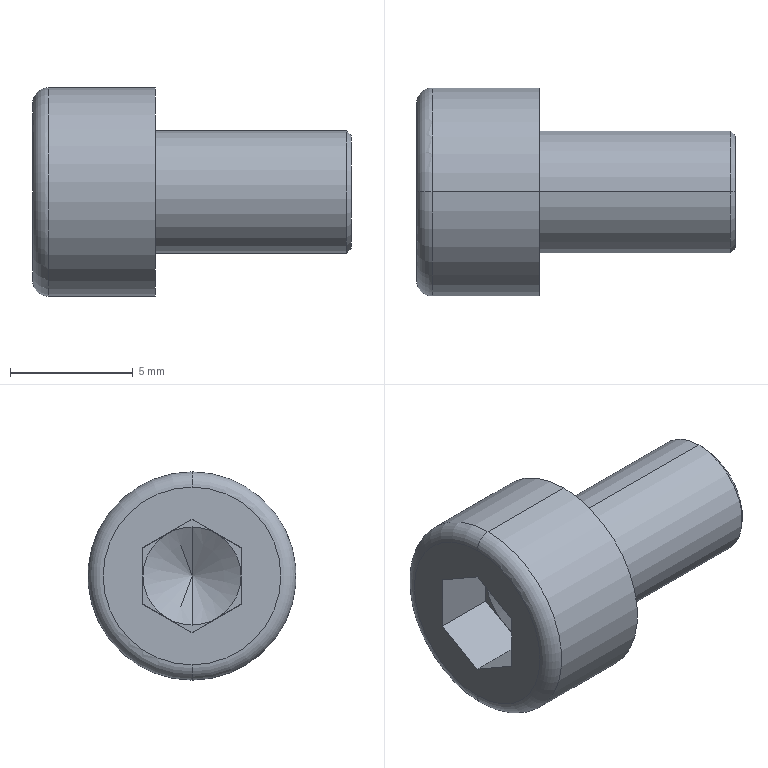Part | STEP file | hexagon socket head cap screws gb_GB_FASTENER_SCREWS_HSHCS M5X8-C | 1 solid | 25 faces | box 13 x 8.5 x 8.5 mm | volume 398.856 mm3 | plane 15 | cone 4 | cylinder 4 | torus 2 | commonest cylinder face diameters 5 x2 8.5 x2
STEP:
#1=CARTESIAN_POINT('',(13.,0.,-2.3));
#2=VERTEX_POINT('',#1);
#3=CARTESIAN_POINT('',(13.,0.,2.3));
#4=VERTEX_POINT('',#3);
#5=CARTESIAN_POINT('',(13.,0.,0.));
#6=DIRECTION('',(1.,0.,0.));
#7=DIRECTION('',(0.,0.,-1.));
#8=AXIS2_PLACEMENT_3D('',#5,#6,#7);
#9=CIRCLE('',#8,2.3);
#10=EDGE_CURVE('',#2,#4,#9,.T.);
#11=ORIENTED_EDGE('',*,*,#10,.F.);
#12=CARTESIAN_POINT('',(12.8,0.,-2.5));
#13=VERTEX_POINT('',#12);
#14=CARTESIAN_POINT('',(13.,0.,-2.3));
#15=DIRECTION('',(-0.7071,0.,-0.7071));
#16=VECTOR('',#15,1000.);
#17=LINE('',#14,#16);
#18=EDGE_CURVE('',#2,#13,#17,.T.);
#19=ORIENTED_EDGE('',*,*,#18,.T.);
#20=CARTESIAN_POINT('',(12.8,0.,2.5));
#21=VERTEX_POINT('',#20);
#22=CARTESIAN_POINT('',(12.8,0.,0.));
#23=DIRECTION('',(-1.,0.,0.));
#24=DIRECTION('',(0.,0.,-1.));
#25=AXIS2_PLACEMENT_3D('',#22,#23,#24);
#26=CIRCLE('',#25,2.5);
#27=EDGE_CURVE('',#21,#13,#26,.T.);
#28=ORIENTED_EDGE('',*,*,#27,.F.);
#29=CARTESIAN_POINT('',(13.,0.,2.3));
#30=DIRECTION('',(-0.7071,0.,0.7071));
#31=VECTOR('',#30,1000.);
#32=LINE('',#29,#31);
#33=EDGE_CURVE('',#4,#21,#32,.T.);
#34=ORIENTED_EDGE('',*,*,#33,.F.);
#35=EDGE_LOOP('',(#11,#19,#28,#34));
#36=FACE_OUTER_BOUND('',#35,.T.);
#37=CARTESIAN_POINT('',(13.,0.,0.));
#38=DIRECTION('',(-1.,0.,0.));
#39=DIRECTION('',(0.,0.,1.));
#40=AXIS2_PLACEMENT_3D('',#37,#38,#39);
#41=CONICAL_SURFACE('',#40,2.3,0.7854);
#42=ADVANCED_FACE('',(#36),#41,.T.);
#43=CARTESIAN_POINT('',(0.,0.,3.625));
#44=VERTEX_POINT('',#43);
#45=CARTESIAN_POINT('',(0.,0.,-3.625));
#46=VERTEX_POINT('',#45);
#47=CARTESIAN_POINT('',(0.,0.,0.));
#48=DIRECTION('',(-1.,0.,0.));
#49=DIRECTION('',(0.,0.,-1.));
#50=AXIS2_PLACEMENT_3D('',#47,#48,#49);
#51=CIRCLE('',#50,3.625);
#52=EDGE_CURVE('',#44,#46,#51,.T.);
#53=ORIENTED_EDGE('',*,*,#52,.F.);
#54=CARTESIAN_POINT('',(0.625,0.,4.25));
#55=VERTEX_POINT('',#54);
#56=CARTESIAN_POINT('',(0.625,0.,3.625));
#57=DIRECTION('',(0.,1.,0.));
#58=DIRECTION('',(0.,0.,1.));
#59=AXIS2_PLACEMENT_3D('',#56,#57,#58);
#60=CIRCLE('',#59,0.625);
#61=EDGE_CURVE('',#44,#55,#60,.T.);
#62=ORIENTED_EDGE('',*,*,#61,.T.);
#63=CARTESIAN_POINT('',(0.625,0.,-4.25));
#64=VERTEX_POINT('',#63);
#65=CARTESIAN_POINT('',(0.625,0.,0.));
#66=DIRECTION('',(1.,0.,0.));
#67=DIRECTION('',(0.,0.,-1.));
#68=AXIS2_PLACEMENT_3D('',#65,#66,#67);
#69=CIRCLE('',#68,4.25);
#70=EDGE_CURVE('',#64,#55,#69,.T.);
#71=ORIENTED_EDGE('',*,*,#70,.F.);
#72=CARTESIAN_POINT('',(0.625,0.,-3.625));
#73=DIRECTION('',(0.,-1.,0.));
#74=DIRECTION('',(0.,0.,-1.));
#75=AXIS2_PLACEMENT_3D('',#72,#73,#74);
#76=CIRCLE('',#75,0.625);
#77=EDGE_CURVE('',#46,#64,#76,.T.);
#78=ORIENTED_EDGE('',*,*,#77,.F.);
#79=EDGE_LOOP('',(#53,#62,#71,#78));
#80=FACE_OUTER_BOUND('',#79,.T.);
#81=CARTESIAN_POINT('',(0.625,0.,0.));
#82=DIRECTION('',(1.,0.,0.));
#83=DIRECTION('',(0.,0.,-1.));
#84=AXIS2_PLACEMENT_3D('',#81,#82,#83);
#85=TOROIDAL_SURFACE('',#84,3.625,0.625);
#86=ADVANCED_FACE('',(#80),#85,.T.);
#87=CARTESIAN_POINT('',(3.655,0.,0.));
#88=VERTEX_POINT('',#87);
#89=CARTESIAN_POINT('',(2.5,0.,2.));
#90=VERTEX_POINT('',#89);
#91=CARTESIAN_POINT('',(2.5,0.,2.));
#92=DIRECTION('',(-0.5,0.,0.866));
#93=VECTOR('',#92,1000.);
#94=LINE('',#91,#93);
#95=EDGE_CURVE('',#88,#90,#94,.T.);
#96=ORIENTED_EDGE('',*,*,#95,.F.);
#97=CARTESIAN_POINT('',(2.5,0.,-2.));
#98=VERTEX_POINT('',#97);
#99=CARTESIAN_POINT('',(2.5,0.,-2.));
#100=DIRECTION('',(-0.5,0.,-0.866));
#101=VECTOR('',#100,1000.);
#102=LINE('',#99,#101);
#103=EDGE_CURVE('',#88,#98,#102,.T.);
#104=ORIENTED_EDGE('',*,*,#103,.T.);
#105=CARTESIAN_POINT('',(2.5,-1.,-1.732));
#106=VERTEX_POINT('',#105);
#107=CARTESIAN_POINT('',(2.5,0.,0.));
#108=DIRECTION('',(-1.,0.,0.));
#109=DIRECTION('',(0.,0.,-1.));
#110=AXIS2_PLACEMENT_3D('',#107,#108,#109);
#111=CIRCLE('',#110,2.);
#112=EDGE_CURVE('',#98,#106,#111,.T.);
#113=ORIENTED_EDGE('',*,*,#112,.T.);
#114=CARTESIAN_POINT('',(2.5,-2.,0.));
#115=VERTEX_POINT('',#114);
#116=CARTESIAN_POINT('',(2.5,0.,0.));
#117=DIRECTION('',(-1.,0.,0.));
#118=DIRECTION('',(0.,0.,-1.));
#119=AXIS2_PLACEMENT_3D('',#116,#117,#118);
#120=CIRCLE('',#119,2.);
#121=EDGE_CURVE('',#106,#115,#120,.T.);
#122=ORIENTED_EDGE('',*,*,#121,.T.);
#123=CARTESIAN_POINT('',(2.5,-1.,1.732));
#124=VERTEX_POINT('',#123);
#125=CARTESIAN_POINT('',(2.5,0.,0.));
#126=DIRECTION('',(-1.,0.,0.));
#127=DIRECTION('',(0.,0.,-1.));
#128=AXIS2_PLACEMENT_3D('',#125,#126,#127);
#129=CIRCLE('',#128,2.);
#130=EDGE_CURVE('',#115,#124,#129,.T.);
#131=ORIENTED_EDGE('',*,*,#130,.T.);
#132=CARTESIAN_POINT('',(2.5,0.,0.));
#133=DIRECTION('',(-1.,0.,0.));
#134=DIRECTION('',(0.,0.,-1.));
#135=AXIS2_PLACEMENT_3D('',#132,#133,#134);
#136=CIRCLE('',#135,2.);
#137=EDGE_CURVE('',#124,#90,#136,.T.);
#138=ORIENTED_EDGE('',*,*,#137,.T.);
#139=EDGE_LOOP('',(#96,#104,#113,#122,#131,#138));
#140=FACE_OUTER_BOUND('',#139,.T.);
#141=CARTESIAN_POINT('',(2.5,0.,0.));
#142=DIRECTION('',(-1.,0.,0.));
#143=DIRECTION('',(0.,0.,1.));
#144=AXIS2_PLACEMENT_3D('',#141,#142,#143);
#145=CONICAL_SURFACE('',#144,2.,1.047);
#146=ADVANCED_FACE('',(#140),#145,.F.);
#147=ORIENTED_EDGE('',*,*,#27,.T.);
#148=CARTESIAN_POINT('',(5.,0.,-2.5));
#149=VERTEX_POINT('',#148);
#150=CARTESIAN_POINT('',(13.,0.,-2.5));
#151=DIRECTION('',(-1.,0.,0.));
#152=VECTOR('',#151,1000.);
#153=LINE('',#150,#152);
#154=EDGE_CURVE('',#13,#149,#153,.T.);
#155=ORIENTED_EDGE('',*,*,#154,.T.);
#156=CARTESIAN_POINT('',(5.,0.,2.5));
#157=VERTEX_POINT('',#156);
#158=CARTESIAN_POINT('',(5.,0.,0.));
#159=DIRECTION('',(1.,0.,0.));
#160=DIRECTION('',(0.,0.,-1.));
#161=AXIS2_PLACEMENT_3D('',#158,#159,#160);
#162=CIRCLE('',#161,2.5);
#163=EDGE_CURVE('',#149,#157,#162,.T.);
#164=ORIENTED_EDGE('',*,*,#163,.T.);
#165=CARTESIAN_POINT('',(13.,0.,2.5));
#166=DIRECTION('',(-1.,0.,0.));
#167=VECTOR('',#166,1000.);
#168=LINE('',#165,#167);
#169=EDGE_CURVE('',#21,#157,#168,.T.);
#170=ORIENTED_EDGE('',*,*,#169,.F.);
#171=EDGE_LOOP('',(#147,#155,#164,#170));
#172=FACE_OUTER_BOUND('',#171,.T.);
#173=CARTESIAN_POINT('',(13.,0.,0.));
#174=DIRECTION('',(-1.,0.,0.));
#175=DIRECTION('',(0.,0.,1.));
#176=AXIS2_PLACEMENT_3D('',#173,#174,#175);
#177=CYLINDRICAL_SURFACE('',#176,2.5);
#178=ADVANCED_FACE('',(#172),#177,.T.);
#179=CARTESIAN_POINT('',(5.,0.,-4.25));
#180=VERTEX_POINT('',#179);
#181=CARTESIAN_POINT('',(5.,0.,4.25));
#182=VERTEX_POINT('',#181);
#183=CARTESIAN_POINT('',(5.,0.,0.));
#184=DIRECTION('',(1.,0.,0.));
#185=DIRECTION('',(0.,0.,-1.));
#186=AXIS2_PLACEMENT_3D('',#183,#184,#185);
#187=CIRCLE('',#186,4.25);
#188=EDGE_CURVE('',#180,#182,#187,.T.);
#189=ORIENTED_EDGE('',*,*,#188,.F.);
#190=CARTESIAN_POINT('',(5.,0.,-4.25));
#191=DIRECTION('',(-1.,0.,0.));
#192=VECTOR('',#191,1000.);
#193=LINE('',#190,#192);
#194=EDGE_CURVE('',#180,#64,#193,.T.);
#195=ORIENTED_EDGE('',*,*,#194,.T.);
#196=ORIENTED_EDGE('',*,*,#70,.T.);
#197=CARTESIAN_POINT('',(5.,0.,4.25));
#198=DIRECTION('',(-1.,0.,0.));
#199=VECTOR('',#198,1000.);
#200=LINE('',#197,#199);
#201=EDGE_CURVE('',#182,#55,#200,.T.);
#202=ORIENTED_EDGE('',*,*,#201,.F.);
#203=EDGE_LOOP('',(#189,#195,#196,#202));
#204=FACE_OUTER_BOUND('',#203,.T.);
#205=CARTESIAN_POINT('',(5.,0.,0.));
#206=DIRECTION('',(-1.,0.,0.));
#207=DIRECTION('',(0.,0.,1.));
#208=AXIS2_PLACEMENT_3D('',#205,#206,#207);
#209=CYLINDRICAL_SURFACE('',#208,4.25);
#210=ADVANCED_FACE('',(#204),#209,.T.);
#211=ORIENTED_EDGE('',*,*,#121,.F.);
#212=CARTESIAN_POINT('',(2.5,-2.,-1.155));
#213=VERTEX_POINT('',#212);
#214=CARTESIAN_POINT('',(2.5,-2.,-1.155));
#215=DIRECTION('',(0.,0.866,-0.5));
#216=VECTOR('',#215,1000.);
#217=LINE('',#214,#216);
#218=EDGE_CURVE('',#213,#106,#217,.T.);
#219=ORIENTED_EDGE('',*,*,#218,.F.);
#220=CARTESIAN_POINT('',(2.5,-2.,1.155));
#221=DIRECTION('',(0.,0.,-1.));
#222=VECTOR('',#221,1000.);
#223=LINE('',#220,#222);
#224=EDGE_CURVE('',#115,#213,#223,.T.);
#225=ORIENTED_EDGE('',*,*,#224,.F.);
#226=EDGE_LOOP('',(#211,#219,#225));
#227=FACE_OUTER_BOUND('',#226,.T.);
#228=CARTESIAN_POINT('',(2.5,0.,-2.309));
#229=DIRECTION('',(1.,0.,0.));
#230=DIRECTION('',(0.,0.,-1.));
#231=AXIS2_PLACEMENT_3D('',#228,#229,#230);
#232=PLANE('',#231);
#233=ADVANCED_FACE('',(#227),#232,.F.);
#234=ORIENTED_EDGE('',*,*,#130,.F.);
#235=CARTESIAN_POINT('',(2.5,-2.,1.155));
#236=VERTEX_POINT('',#235);
#237=CARTESIAN_POINT('',(2.5,-2.,1.155));
#238=DIRECTION('',(0.,0.,-1.));
#239=VECTOR('',#238,1000.);
#240=LINE('',#237,#239);
#241=EDGE_CURVE('',#236,#115,#240,.T.);
#242=ORIENTED_EDGE('',*,*,#241,.F.);
#243=CARTESIAN_POINT('',(2.5,0.,2.309));
#244=DIRECTION('',(0.,-0.866,-0.5));
#245=VECTOR('',#244,1000.);
#246=LINE('',#243,#245);
#247=EDGE_CURVE('',#124,#236,#246,.T.);
#248=ORIENTED_EDGE('',*,*,#247,.F.);
#249=EDGE_LOOP('',(#234,#242,#248));
#250=FACE_OUTER_BOUND('',#249,.T.);
#251=CARTESIAN_POINT('',(2.5,0.,-2.309));
#252=DIRECTION('',(1.,0.,0.));
#253=DIRECTION('',(0.,0.,-1.));
#254=AXIS2_PLACEMENT_3D('',#251,#252,#253);
#255=PLANE('',#254);
#256=ADVANCED_FACE('',(#250),#255,.F.);
#257=ORIENTED_EDGE('',*,*,#137,.F.);
#258=CARTESIAN_POINT('',(2.5,0.,2.309));
#259=VERTEX_POINT('',#258);
#260=CARTESIAN_POINT('',(2.5,0.,2.309));
#261=DIRECTION('',(0.,-0.866,-0.5));
#262=VECTOR('',#261,1000.);
#263=LINE('',#260,#262);
#264=EDGE_CURVE('',#259,#124,#263,.T.);
#265=ORIENTED_EDGE('',*,*,#264,.F.);
#266=CARTESIAN_POINT('',(2.5,1.,1.732));
#267=VERTEX_POINT('',#266);
#268=CARTESIAN_POINT('',(2.5,2.,1.155));
#269=DIRECTION('',(0.,-0.866,0.5));
#270=VECTOR('',#269,1000.);
#271=LINE('',#268,#270);
#272=EDGE_CURVE('',#267,#259,#271,.T.);
#273=ORIENTED_EDGE('',*,*,#272,.F.);
#274=CARTESIAN_POINT('',(2.5,0.,0.));
#275=DIRECTION('',(-1.,0.,0.));
#276=DIRECTION('',(0.,0.,-1.));
#277=AXIS2_PLACEMENT_3D('',#274,#275,#276);
#278=CIRCLE('',#277,2.);
#279=EDGE_CURVE('',#90,#267,#278,.T.);
#280=ORIENTED_EDGE('',*,*,#279,.F.);
#281=EDGE_LOOP('',(#257,#265,#273,#280));
#282=FACE_OUTER_BOUND('',#281,.T.);
#283=CARTESIAN_POINT('',(2.5,0.,-2.309));
#284=DIRECTION('',(1.,0.,0.));
#285=DIRECTION('',(0.,0.,-1.));
#286=AXIS2_PLACEMENT_3D('',#283,#284,#285);
#287=PLANE('',#286);
#288=ADVANCED_FACE('',(#282),#287,.F.);
#289=CARTESIAN_POINT('',(2.5,2.,0.));
#290=VERTEX_POINT('',#289);
#291=CARTESIAN_POINT('',(2.5,0.,0.));
#292=DIRECTION('',(-1.,0.,0.));
#293=DIRECTION('',(0.,0.,-1.));
#294=AXIS2_PLACEMENT_3D('',#291,#292,#293);
#295=CIRCLE('',#294,2.);
#296=EDGE_CURVE('',#267,#290,#295,.T.);
#297=ORIENTED_EDGE('',*,*,#296,.F.);
#298=CARTESIAN_POINT('',(2.5,2.,1.155));
#299=VERTEX_POINT('',#298);
#300=CARTESIAN_POINT('',(2.5,2.,1.155));
#301=DIRECTION('',(0.,-0.866,0.5));
#302=VECTOR('',#301,1000.);
#303=LINE('',#300,#302);
#304=EDGE_CURVE('',#299,#267,#303,.T.);
#305=ORIENTED_EDGE('',*,*,#304,.F.);
#306=CARTESIAN_POINT('',(2.5,2.,-1.155));
#307=DIRECTION('',(0.,0.,1.));
#308=VECTOR('',#307,1000.);
#309=LINE('',#306,#308);
#310=EDGE_CURVE('',#290,#299,#309,.T.);
#311=ORIENTED_EDGE('',*,*,#310,.F.);
#312=EDGE_LOOP('',(#297,#305,#311));
#313=FACE_OUTER_BOUND('',#312,.T.);
#314=CARTESIAN_POINT('',(2.5,0.,-2.309));
#315=DIRECTION('',(1.,0.,0.));
#316=DIRECTION('',(0.,0.,-1.));
#317=AXIS2_PLACEMENT_3D('',#314,#315,#316);
#318=PLANE('',#317);
#319=ADVANCED_FACE('',(#313),#318,.F.);
#320=CARTESIAN_POINT('',(2.5,1.,-1.732));
#321=VERTEX_POINT('',#320);
#322=CARTESIAN_POINT('',(2.5,0.,0.));
#323=DIRECTION('',(1.,0.,0.));
#324=DIRECTION('',(0.,0.,-1.));
#325=AXIS2_PLACEMENT_3D('',#322,#323,#324);
#326=CIRCLE('',#325,2.);
#327=EDGE_CURVE('',#321,#290,#326,.T.);
#328=ORIENTED_EDGE('',*,*,#327,.T.);
#329=CARTESIAN_POINT('',(2.5,2.,-1.155));
#330=VERTEX_POINT('',#329);
#331=CARTESIAN_POINT('',(2.5,2.,-1.155));
#332=DIRECTION('',(0.,0.,1.));
#333=VECTOR('',#332,1000.);
#334=LINE('',#331,#333);
#335=EDGE_CURVE('',#330,#290,#334,.T.);
#336=ORIENTED_EDGE('',*,*,#335,.F.);
#337=CARTESIAN_POINT('',(2.5,0.,-2.309));
#338=DIRECTION('',(0.,0.866,0.5));
#339=VECTOR('',#338,1000.);
#340=LINE('',#337,#339);
#341=EDGE_CURVE('',#321,#330,#340,.T.);
#342=ORIENTED_EDGE('',*,*,#341,.F.);
#343=EDGE_LOOP('',(#328,#336,#342));
#344=FACE_OUTER_BOUND('',#343,.T.);
#345=CARTESIAN_POINT('',(2.5,0.,-2.309));
#346=DIRECTION('',(1.,0.,0.));
#347=DIRECTION('',(0.,0.,-1.));
#348=AXIS2_PLACEMENT_3D('',#345,#346,#347);
#349=PLANE('',#348);
#350=ADVANCED_FACE('',(#344),#349,.F.);
#351=CARTESIAN_POINT('',(2.5,0.,0.));
#352=DIRECTION('',(-1.,0.,0.));
#353=DIRECTION('',(0.,0.,-1.));
#354=AXIS2_PLACEMENT_3D('',#351,#352,#353);
#355=CIRCLE('',#354,2.);
#356=EDGE_CURVE('',#321,#98,#355,.T.);
#357=ORIENTED_EDGE('',*,*,#356,.F.);
#358=CARTESIAN_POINT('',(2.5,0.,-2.309));
#359=VERTEX_POINT('',#358);
#360=CARTESIAN_POINT('',(2.5,0.,-2.309));
#361=DIRECTION('',(0.,0.866,0.5));
#362=VECTOR('',#361,1000.);
#363=LINE('',#360,#362);
#364=EDGE_CURVE('',#359,#321,#363,.T.);
#365=ORIENTED_EDGE('',*,*,#364,.F.);
#366=CARTESIAN_POINT('',(2.5,-2.,-1.155));
#367=DIRECTION('',(0.,0.866,-0.5));
#368=VECTOR('',#367,1000.);
#369=LINE('',#366,#368);
#370=EDGE_CURVE('',#106,#359,#369,.T.);
#371=ORIENTED_EDGE('',*,*,#370,.F.);
#372=ORIENTED_EDGE('',*,*,#112,.F.);
#373=EDGE_LOOP('',(#357,#365,#371,#372));
#374=FACE_OUTER_BOUND('',#373,.T.);
#375=CARTESIAN_POINT('',(2.5,0.,-2.309));
#376=DIRECTION('',(1.,0.,0.));
#377=DIRECTION('',(0.,0.,-1.));
#378=AXIS2_PLACEMENT_3D('',#375,#376,#377);
#379=PLANE('',#378);
#380=ADVANCED_FACE('',(#374),#379,.F.);
#381=CARTESIAN_POINT('',(0.,0.,0.));
#382=DIRECTION('',(-1.,0.,0.));
#383=DIRECTION('',(0.,0.,-1.));
#384=AXIS2_PLACEMENT_3D('',#381,#382,#383);
#385=CIRCLE('',#384,3.625);
#386=EDGE_CURVE('',#46,#44,#385,.T.);
#387=ORIENTED_EDGE('',*,*,#386,.T.);
#388=ORIENTED_EDGE('',*,*,#52,.T.);
#389=EDGE_LOOP('',(#387,#388));
#390=FACE_OUTER_BOUND('',#389,.T.);
#391=CARTESIAN_POINT('',(0.,-2.,-1.155));
#392=VERTEX_POINT('',#391);
#393=CARTESIAN_POINT('',(0.,0.,-2.309));
#394=VERTEX_POINT('',#393);
#395=CARTESIAN_POINT('',(0.,-2.,-1.155));
#396=DIRECTION('',(0.,0.866,-0.5));
#397=VECTOR('',#396,1000.);
#398=LINE('',#395,#397);
#399=EDGE_CURVE('',#392,#394,#398,.T.);
#400=ORIENTED_EDGE('',*,*,#399,.T.);
#401=CARTESIAN_POINT('',(0.,2.,-1.155));
#402=VERTEX_POINT('',#401);
#403=CARTESIAN_POINT('',(0.,0.,-2.309));
#404=DIRECTION('',(0.,0.866,0.5));
#405=VECTOR('',#404,1000.);
#406=LINE('',#403,#405);
#407=EDGE_CURVE('',#394,#402,#406,.T.);
#408=ORIENTED_EDGE('',*,*,#407,.T.);
#409=CARTESIAN_POINT('',(0.,2.,1.155));
#410=VERTEX_POINT('',#409);
#411=CARTESIAN_POINT('',(0.,2.,-1.155));
#412=DIRECTION('',(0.,0.,1.));
#413=VECTOR('',#412,1000.);
#414=LINE('',#411,#413);
#415=EDGE_CURVE('',#402,#410,#414,.T.);
#416=ORIENTED_EDGE('',*,*,#415,.T.);
#417=CARTESIAN_POINT('',(0.,0.,2.309));
#418=VERTEX_POINT('',#417);
#419=CARTESIAN_POINT('',(0.,2.,1.155));
#420=DIRECTION('',(0.,-0.866,0.5));
#421=VECTOR('',#420,1000.);
#422=LINE('',#419,#421);
#423=EDGE_CURVE('',#410,#418,#422,.T.);
#424=ORIENTED_EDGE('',*,*,#423,.T.);
#425=CARTESIAN_POINT('',(0.,-2.,1.155));
#426=VERTEX_POINT('',#425);
#427=CARTESIAN_POINT('',(0.,0.,2.309));
#428=DIRECTION('',(0.,-0.866,-0.5));
#429=VECTOR('',#428,1000.);
#430=LINE('',#427,#429);
#431=EDGE_CURVE('',#418,#426,#430,.T.);
#432=ORIENTED_EDGE('',*,*,#431,.T.);
#433=CARTESIAN_POINT('',(0.,-2.,1.155));
#434=DIRECTION('',(0.,0.,-1.));
#435=VECTOR('',#434,1000.);
#436=LINE('',#433,#435);
#437=EDGE_CURVE('',#426,#392,#436,.T.);
#438=ORIENTED_EDGE('',*,*,#437,.T.);
#439=EDGE_LOOP('',(#400,#408,#416,#424,#432,#438));
#440=FACE_BOUND('',#439,.T.);
#441=CARTESIAN_POINT('',(0.,0.,0.));
#442=DIRECTION('',(1.,0.,0.));
#443=DIRECTION('',(0.,0.,-1.));
#444=AXIS2_PLACEMENT_3D('',#441,#442,#443);
#445=PLANE('',#444);
#446=ADVANCED_FACE('',(#390,#440),#445,.F.);
#447=CARTESIAN_POINT('',(5.,0.,0.));
#448=DIRECTION('',(1.,0.,0.));
#449=DIRECTION('',(0.,0.,-1.));
#450=AXIS2_PLACEMENT_3D('',#447,#448,#449);
#451=CIRCLE('',#450,4.25);
#452=EDGE_CURVE('',#182,#180,#451,.T.);
#453=ORIENTED_EDGE('',*,*,#452,.T.);
#454=ORIENTED_EDGE('',*,*,#188,.T.);
#455=EDGE_LOOP('',(#453,#454));
#456=FACE_OUTER_BOUND('',#455,.T.);
#457=CARTESIAN_POINT('',(5.,0.,0.));
#458=DIRECTION('',(1.,0.,0.));
#459=DIRECTION('',(0.,0.,-1.));
#460=AXIS2_PLACEMENT_3D('',#457,#458,#459);
#461=CIRCLE('',#460,2.5);
#462=EDGE_CURVE('',#157,#149,#461,.T.);
#463=ORIENTED_EDGE('',*,*,#462,.F.);
#464=ORIENTED_EDGE('',*,*,#163,.F.);
#465=EDGE_LOOP('',(#463,#464));
#466=FACE_BOUND('',#465,.T.);
#467=CARTESIAN_POINT('',(5.,0.,0.));
#468=DIRECTION('',(1.,0.,0.));
#469=DIRECTION('',(0.,0.,-1.));
#470=AXIS2_PLACEMENT_3D('',#467,#468,#469);
#471=PLANE('',#470);
#472=ADVANCED_FACE('',(#456,#466),#471,.T.);
#473=ORIENTED_EDGE('',*,*,#194,.F.);
#474=ORIENTED_EDGE('',*,*,#452,.F.);
#475=ORIENTED_EDGE('',*,*,#201,.T.);
#476=CARTESIAN_POINT('',(0.625,0.,0.));
#477=DIRECTION('',(1.,0.,0.));
#478=DIRECTION('',(0.,0.,-1.));
#479=AXIS2_PLACEMENT_3D('',#476,#477,#478);
#480=CIRCLE('',#479,4.25);
#481=EDGE_CURVE('',#55,#64,#480,.T.);
#482=ORIENTED_EDGE('',*,*,#481,.T.);
#483=EDGE_LOOP('',(#473,#474,#475,#482));
#484=FACE_OUTER_BOUND('',#483,.T.);
#485=CARTESIAN_POINT('',(5.,0.,0.));
#486=DIRECTION('',(-1.,0.,0.));
#487=DIRECTION('',(0.,0.,1.));
#488=AXIS2_PLACEMENT_3D('',#485,#486,#487);
#489=CYLINDRICAL_SURFACE('',#488,4.25);
#490=ADVANCED_FACE('',(#484),#489,.T.);
#491=ORIENTED_EDGE('',*,*,#154,.F.);
#492=CARTESIAN_POINT('',(12.8,0.,0.));
#493=DIRECTION('',(-1.,0.,0.));
#494=DIRECTION('',(0.,0.,-1.));
#495=AXIS2_PLACEMENT_3D('',#492,#493,#494);
#496=CIRCLE('',#495,2.5);
#497=EDGE_CURVE('',#13,#21,#496,.T.);
#498=ORIENTED_EDGE('',*,*,#497,.T.);
#499=ORIENTED_EDGE('',*,*,#169,.T.);
#500=ORIENTED_EDGE('',*,*,#462,.T.);
#501=EDGE_LOOP('',(#491,#498,#499,#500));
#502=FACE_OUTER_BOUND('',#501,.T.);
#503=CARTESIAN_POINT('',(13.,0.,0.));
#504=DIRECTION('',(-1.,0.,0.));
#505=DIRECTION('',(0.,0.,1.));
#506=AXIS2_PLACEMENT_3D('',#503,#504,#505);
#507=CYLINDRICAL_SURFACE('',#506,2.5);
#508=ADVANCED_FACE('',(#502),#507,.T.);
#509=CARTESIAN_POINT('',(13.,0.,0.));
#510=DIRECTION('',(1.,0.,0.));
#511=DIRECTION('',(0.,0.,-1.));
#512=AXIS2_PLACEMENT_3D('',#509,#510,#511);
#513=CIRCLE('',#512,2.3);
#514=EDGE_CURVE('',#4,#2,#513,.T.);
#515=ORIENTED_EDGE('',*,*,#514,.T.);
#516=ORIENTED_EDGE('',*,*,#10,.T.);
#517=EDGE_LOOP('',(#515,#516));
#518=FACE_OUTER_BOUND('',#517,.T.);
#519=CARTESIAN_POINT('',(13.,0.,0.));
#520=DIRECTION('',(1.,0.,0.));
#521=DIRECTION('',(0.,0.,-1.));
#522=AXIS2_PLACEMENT_3D('',#519,#520,#521);
#523=PLANE('',#522);
#524=ADVANCED_FACE('',(#518),#523,.T.);
#525=ORIENTED_EDGE('',*,*,#399,.F.);
#526=CARTESIAN_POINT('',(2.5,-2.,-1.155));
#527=DIRECTION('',(-1.,0.,0.));
#528=VECTOR('',#527,1000.);
#529=LINE('',#526,#528);
#530=EDGE_CURVE('',#213,#392,#529,.T.);
#531=ORIENTED_EDGE('',*,*,#530,.F.);
#532=ORIENTED_EDGE('',*,*,#218,.T.);
#533=ORIENTED_EDGE('',*,*,#370,.T.);
#534=CARTESIAN_POINT('',(2.5,0.,-2.309));
#535=DIRECTION('',(-1.,0.,0.));
#536=VECTOR('',#535,1000.);
#537=LINE('',#534,#536);
#538=EDGE_CURVE('',#359,#394,#537,.T.);
#539=ORIENTED_EDGE('',*,*,#538,.T.);
#540=EDGE_LOOP('',(#525,#531,#532,#533,#539));
#541=FACE_OUTER_BOUND('',#540,.T.);
#542=CARTESIAN_POINT('',(2.5,-2.,-1.155));
#543=DIRECTION('',(0.,0.5,0.866));
#544=DIRECTION('',(0.,-0.866,0.5));
#545=AXIS2_PLACEMENT_3D('',#542,#543,#544);
#546=PLANE('',#545);
#547=ADVANCED_FACE('',(#541),#546,.T.);
#548=ORIENTED_EDGE('',*,*,#407,.F.);
#549=ORIENTED_EDGE('',*,*,#538,.F.);
#550=ORIENTED_EDGE('',*,*,#364,.T.);
#551=ORIENTED_EDGE('',*,*,#341,.T.);
#552=CARTESIAN_POINT('',(2.5,2.,-1.155));
#553=DIRECTION('',(-1.,0.,0.));
#554=VECTOR('',#553,1000.);
#555=LINE('',#552,#554);
#556=EDGE_CURVE('',#330,#402,#555,.T.);
#557=ORIENTED_EDGE('',*,*,#556,.T.);
#558=EDGE_LOOP('',(#548,#549,#550,#551,#557));
#559=FACE_OUTER_BOUND('',#558,.T.);
#560=CARTESIAN_POINT('',(2.5,0.,-2.309));
#561=DIRECTION('',(0.,-0.5,0.866));
#562=DIRECTION('',(0.,-0.866,-0.5));
#563=AXIS2_PLACEMENT_3D('',#560,#561,#562);
#564=PLANE('',#563);
#565=ADVANCED_FACE('',(#559),#564,.T.);
#566=ORIENTED_EDGE('',*,*,#415,.F.);
#567=ORIENTED_EDGE('',*,*,#556,.F.);
#568=ORIENTED_EDGE('',*,*,#335,.T.);
#569=ORIENTED_EDGE('',*,*,#310,.T.);
#570=CARTESIAN_POINT('',(2.5,2.,1.155));
#571=DIRECTION('',(-1.,0.,0.));
#572=VECTOR('',#571,1000.);
#573=LINE('',#570,#572);
#574=EDGE_CURVE('',#299,#410,#573,.T.);
#575=ORIENTED_EDGE('',*,*,#574,.T.);
#576=EDGE_LOOP('',(#566,#567,#568,#569,#575));
#577=FACE_OUTER_BOUND('',#576,.T.);
#578=CARTESIAN_POINT('',(2.5,2.,-1.155));
#579=DIRECTION('',(0.,-1.,0.));
#580=DIRECTION('',(0.,0.,-1.));
#581=AXIS2_PLACEMENT_3D('',#578,#579,#580);
#582=PLANE('',#581);
#583=ADVANCED_FACE('',(#577),#582,.T.);
#584=ORIENTED_EDGE('',*,*,#423,.F.);
#585=ORIENTED_EDGE('',*,*,#574,.F.);
#586=ORIENTED_EDGE('',*,*,#304,.T.);
#587=ORIENTED_EDGE('',*,*,#272,.T.);
#588=CARTESIAN_POINT('',(2.5,0.,2.309));
#589=DIRECTION('',(-1.,0.,0.));
#590=VECTOR('',#589,1000.);
#591=LINE('',#588,#590);
#592=EDGE_CURVE('',#259,#418,#591,.T.);
#593=ORIENTED_EDGE('',*,*,#592,.T.);
#594=EDGE_LOOP('',(#584,#585,#586,#587,#593));
#595=FACE_OUTER_BOUND('',#594,.T.);
#596=CARTESIAN_POINT('',(2.5,2.,1.155));
#597=DIRECTION('',(0.,-0.5,-0.866));
#598=DIRECTION('',(0.,0.866,-0.5));
#599=AXIS2_PLACEMENT_3D('',#596,#597,#598);
#600=PLANE('',#599);
#601=ADVANCED_FACE('',(#595),#600,.T.);
#602=ORIENTED_EDGE('',*,*,#431,.F.);
#603=ORIENTED_EDGE('',*,*,#592,.F.);
#604=ORIENTED_EDGE('',*,*,#264,.T.);
#605=ORIENTED_EDGE('',*,*,#247,.T.);
#606=CARTESIAN_POINT('',(2.5,-2.,1.155));
#607=DIRECTION('',(-1.,0.,0.));
#608=VECTOR('',#607,1000.);
#609=LINE('',#606,#608);
#610=EDGE_CURVE('',#236,#426,#609,.T.);
#611=ORIENTED_EDGE('',*,*,#610,.T.);
#612=EDGE_LOOP('',(#602,#603,#604,#605,#611));
#613=FACE_OUTER_BOUND('',#612,.T.);
#614=CARTESIAN_POINT('',(2.5,0.,2.309));
#615=DIRECTION('',(0.,0.5,-0.866));
#616=DIRECTION('',(0.,0.866,0.5));
#617=AXIS2_PLACEMENT_3D('',#614,#615,#616);
#618=PLANE('',#617);
#619=ADVANCED_FACE('',(#613),#618,.T.);
#620=ORIENTED_EDGE('',*,*,#437,.F.);
#621=ORIENTED_EDGE('',*,*,#610,.F.);
#622=ORIENTED_EDGE('',*,*,#241,.T.);
#623=ORIENTED_EDGE('',*,*,#224,.T.);
#624=ORIENTED_EDGE('',*,*,#530,.T.);
#625=EDGE_LOOP('',(#620,#621,#622,#623,#624));
#626=FACE_OUTER_BOUND('',#625,.T.);
#627=CARTESIAN_POINT('',(2.5,-2.,1.155));
#628=DIRECTION('',(0.,1.,0.));
#629=DIRECTION('',(0.,0.,1.));
#630=AXIS2_PLACEMENT_3D('',#627,#628,#629);
#631=PLANE('',#630);
#632=ADVANCED_FACE('',(#626),#631,.T.);
#633=ORIENTED_EDGE('',*,*,#103,.F.);
#634=ORIENTED_EDGE('',*,*,#95,.T.);
#635=ORIENTED_EDGE('',*,*,#279,.T.);
#636=ORIENTED_EDGE('',*,*,#296,.T.);
#637=ORIENTED_EDGE('',*,*,#327,.F.);
#638=ORIENTED_EDGE('',*,*,#356,.T.);
#639=EDGE_LOOP('',(#633,#634,#635,#636,#637,#638));
#640=FACE_OUTER_BOUND('',#639,.T.);
#641=CARTESIAN_POINT('',(2.5,0.,0.));
#642=DIRECTION('',(-1.,0.,0.));
#643=DIRECTION('',(0.,0.,1.));
#644=AXIS2_PLACEMENT_3D('',#641,#642,#643);
#645=CONICAL_SURFACE('',#644,2.,1.047);
#646=ADVANCED_FACE('',(#640),#645,.F.);
#647=ORIENTED_EDGE('',*,*,#61,.F.);
#648=ORIENTED_EDGE('',*,*,#386,.F.);
#649=ORIENTED_EDGE('',*,*,#77,.T.);
#650=ORIENTED_EDGE('',*,*,#481,.F.);
#651=EDGE_LOOP('',(#647,#648,#649,#650));
#652=FACE_OUTER_BOUND('',#651,.T.);
#653=CARTESIAN_POINT('',(0.625,0.,0.));
#654=DIRECTION('',(1.,0.,0.));
#655=DIRECTION('',(0.,0.,-1.));
#656=AXIS2_PLACEMENT_3D('',#653,#654,#655);
#657=TOROIDAL_SURFACE('',#656,3.625,0.625);
#658=ADVANCED_FACE('',(#652),#657,.T.);
#659=ORIENTED_EDGE('',*,*,#18,.F.);
#660=ORIENTED_EDGE('',*,*,#514,.F.);
#661=ORIENTED_EDGE('',*,*,#33,.T.);
#662=ORIENTED_EDGE('',*,*,#497,.F.);
#663=EDGE_LOOP('',(#659,#660,#661,#662));
#664=FACE_OUTER_BOUND('',#663,.T.);
#665=CARTESIAN_POINT('',(13.,0.,0.));
#666=DIRECTION('',(-1.,0.,0.));
#667=DIRECTION('',(0.,0.,1.));
#668=AXIS2_PLACEMENT_3D('',#665,#666,#667);
#669=CONICAL_SURFACE('',#668,2.3,0.7854);
#670=ADVANCED_FACE('',(#664),#669,.T.);
#671=CLOSED_SHELL('',(#42,#86,#146,#178,#210,#233,#256,#288,#319,#350,#380,#446,#472,#490,#508,#524,#547,#565,#583,#601,#619,#632,#646,#658,#670));
#672=MANIFOLD_SOLID_BREP('',#671);
#673=CARTESIAN_POINT('',(0.,0.,0.));
#674=DIRECTION('',(0.,0.,1.));
#675=DIRECTION('',(1.,0.,0.));
#676=AXIS2_PLACEMENT_3D('',#673,#674,#675);
#677=(LENGTH_UNIT()NAMED_UNIT(*)SI_UNIT(.MILLI.,.METRE.));
#678=UNCERTAINTY_MEASURE_WITH_UNIT(LENGTH_MEASURE(0.00001),#677,'','');
#679=(NAMED_UNIT(*)PLANE_ANGLE_UNIT()SI_UNIT($,.RADIAN.));
#680=(NAMED_UNIT(*)SI_UNIT($,.STERADIAN.)SOLID_ANGLE_UNIT());
#681=(GEOMETRIC_REPRESENTATION_CONTEXT(3)GLOBAL_UNCERTAINTY_ASSIGNED_CONTEXT((#678))GLOBAL_UNIT_ASSIGNED_CONTEXT((#677,#679,#680))REPRESENTATION_CONTEXT('',''));
#682=ADVANCED_BREP_SHAPE_REPRESENTATION('',(#672,#676),#681);